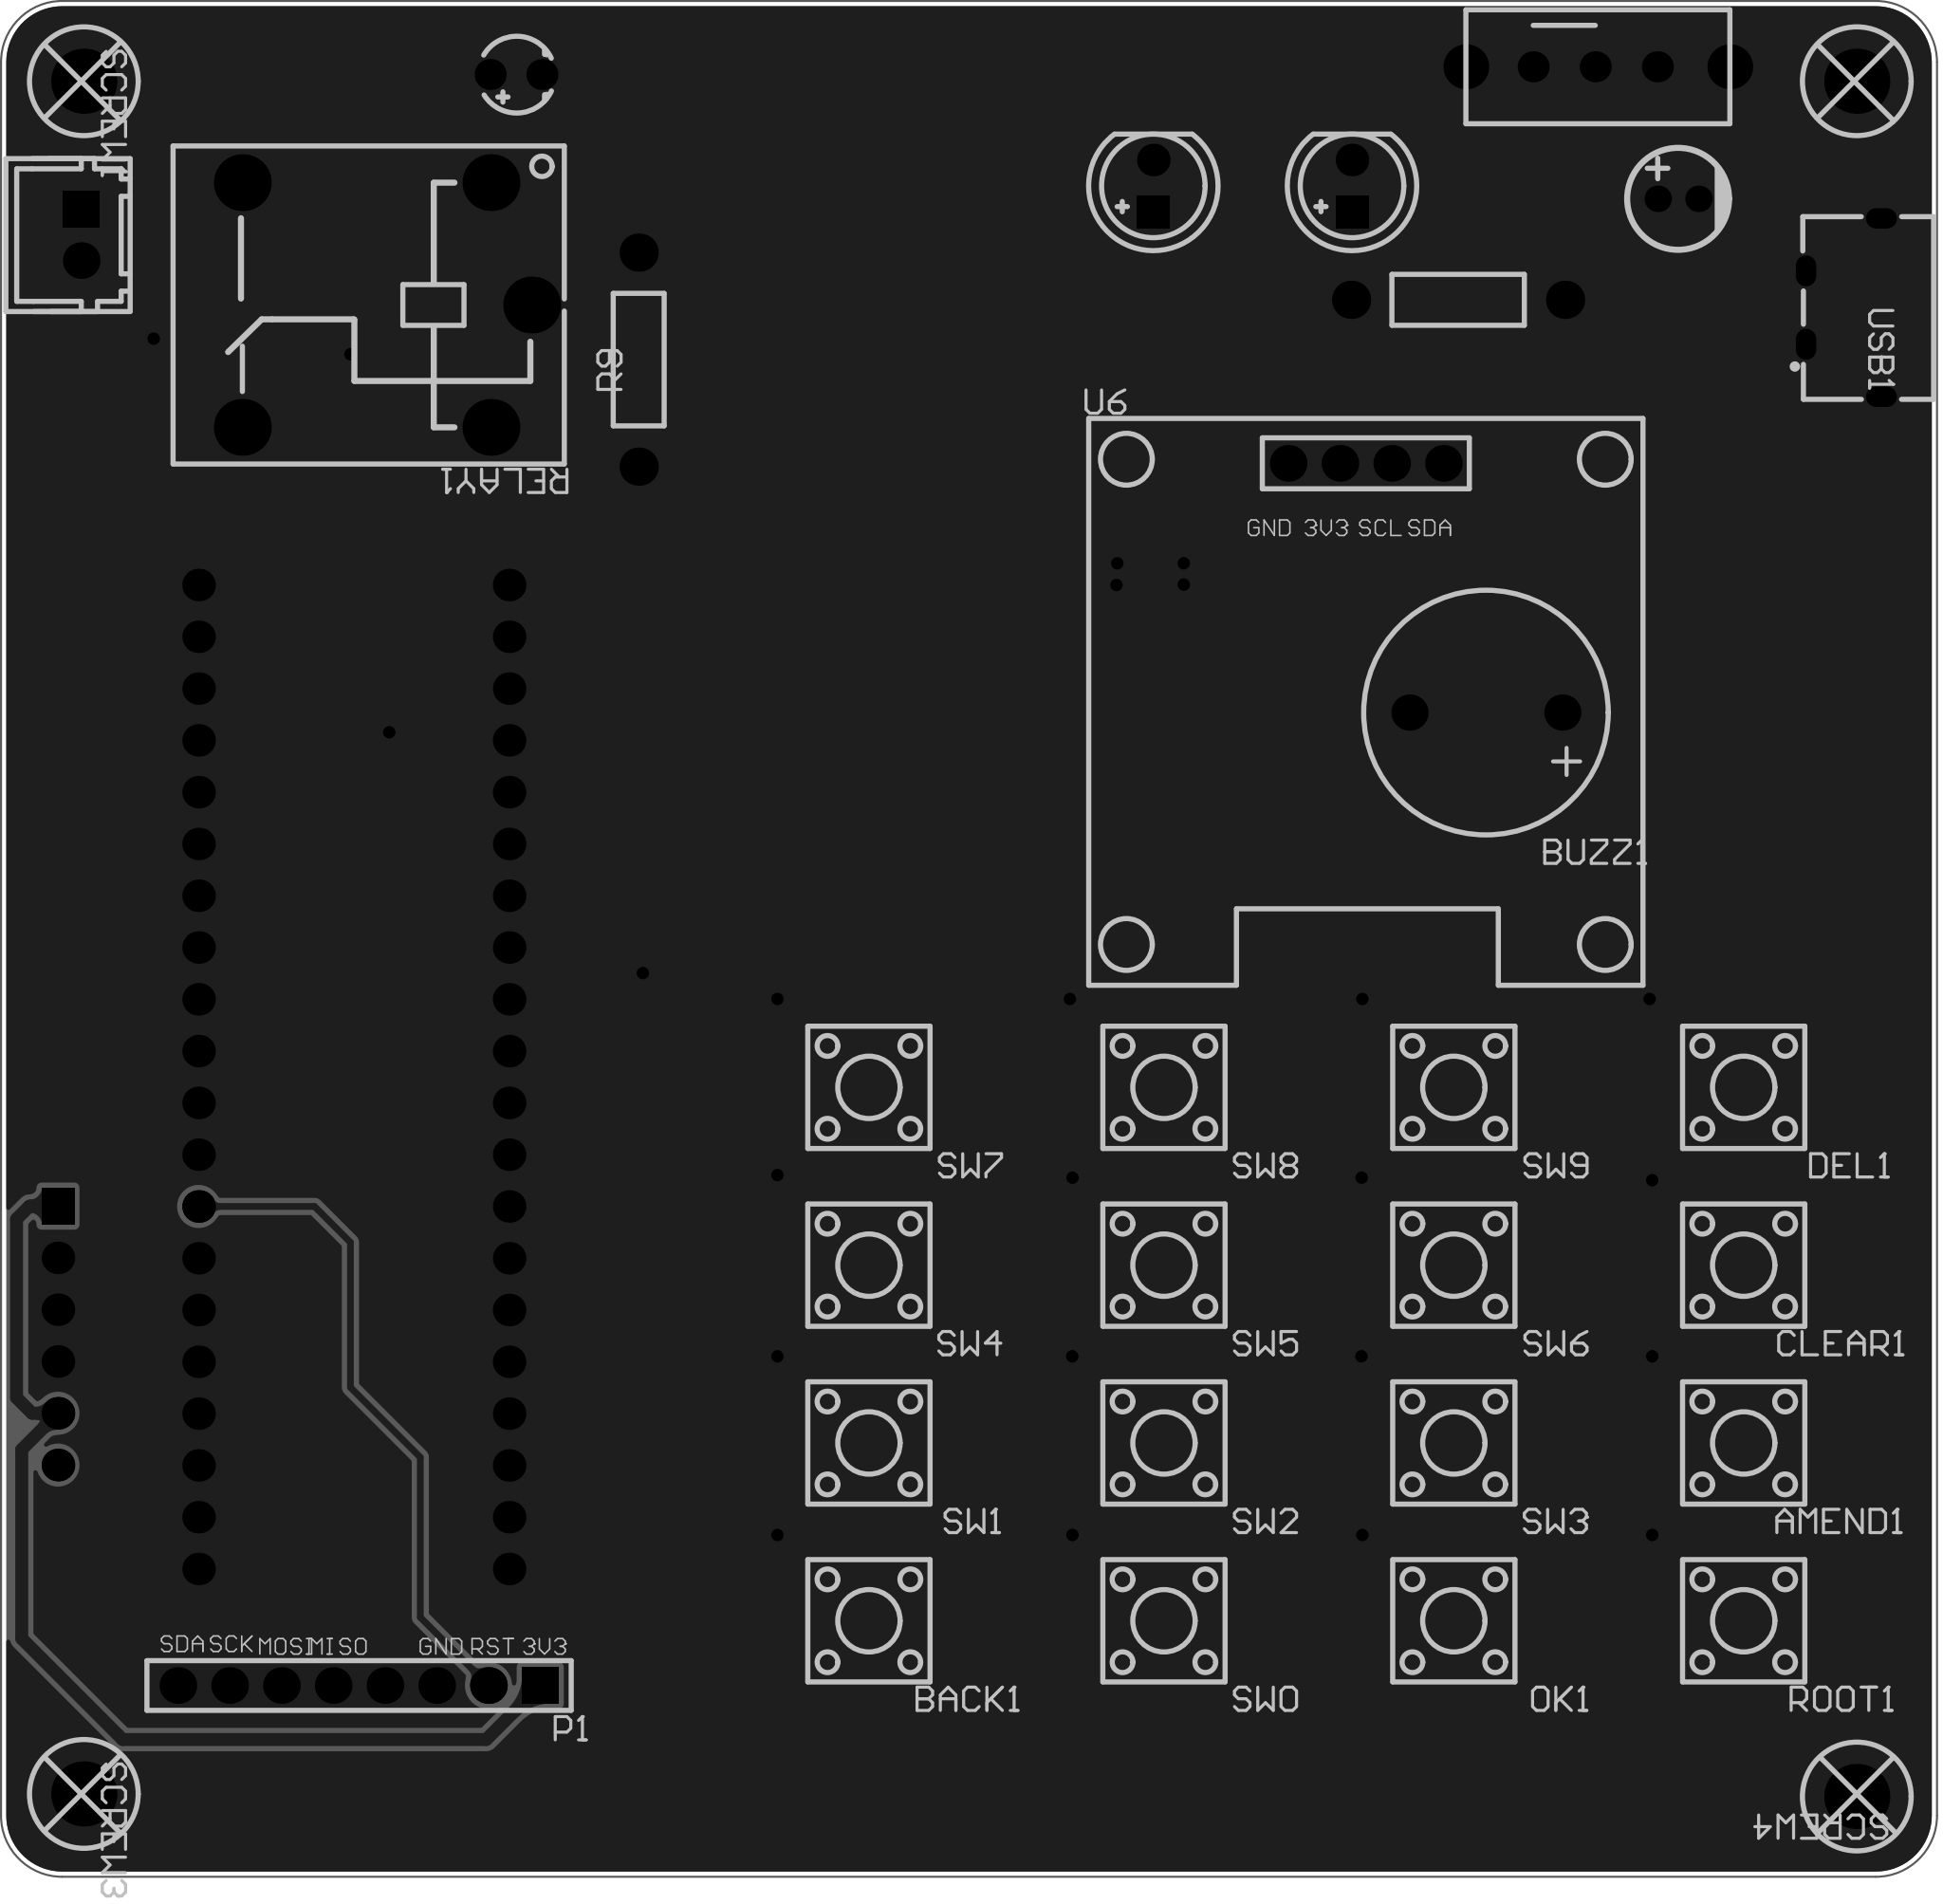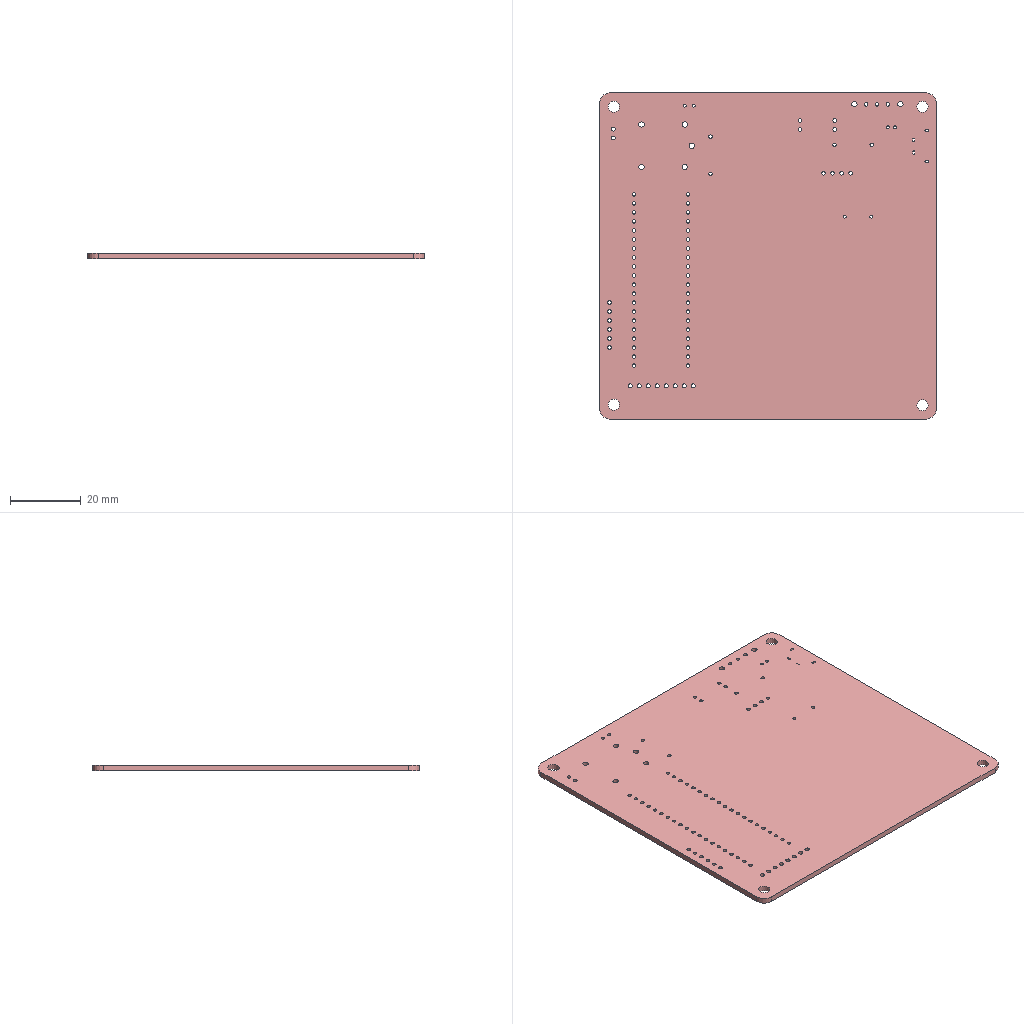Circuit board layout | Altium Designer | box 95 x 92 x 1.6 mm
Layer stack:
# Altium Designer layer stack of  (unit mm; dielectric type: 0 none, 1 core, 2 prepreg, 3 surface material)
index,name,kind,layer,copper_thickness_mm,dielectric_type,dielectric_thickness_mm,dielectric_material,dielectric_constant
0,Top Paste Mask Layer,other,,,,,,
1,Top Silkscreen Layer,other,,,,,,
2,Top Solder Mask Layer,dielectric,,,3,0.01,,3.3
3,Top Layer,copper,Top Layer,0.035,,,,
4,Dielectric1,dielectric,,,3,1.51,FR4,4.5
5,Bottom Layer,copper,Bottom Layer,0.035,,,,
6,Bottom Solder Mask Layer,dielectric,,,3,0.01,,3.3
7,Bottom Silkscreen Layer,other,,,,,,
8,Bottom Paste Mask Layer,other,,,,,,
# drill layer pairs: low layer,high layer
drill_pair,Top Layer,Bottom Layer
Part placement:
Designator,Comment,Layer,Footprint,Center-X(mm),Center-Y(mm),Rotation
BUZZ1,Buzzer BD12.0-P7.50,TopLayer,BUZ-TH_BD12.0-P7.50-D0.6-FD,150.464,138,180
U7,STM32F103C8T6-Card,BottomLayer,CONN-TH_L53.3-W22.9_STM32F103C8T6-CARD,94.912,120.125,90
CN1,ZX-XH2.54-2PZZ,TopLayer,CONN-TH_2P-P2.50_HX25003-2A,81.534,161.417,270
D1,SS14,BottomLayer,SMA_L4.2-W2.6-LS5.3-RD,97.574,154.567,270
RELAY1,SRD-12VDC-SL-C,TopLayer,RELAY-TH_SRD-XXVDC-XL-C,96.539,157.989,180
R1,10.1kΩ,BottomLayer,R0805,126.619,157.837,0
Q1,S8050,BottomLayer,SOT-23-3_L2.9-W1.6-P1.90-LS2.8-BR,93.764,153.17,90
R6,1kΩ,BottomLayer,R0603,92.761,157.107,90
U6,HS96L03W2C03,TopLayer,OLED-TH_L27.8-W27.2-P2.54_C9900033791,144.569,150.224,0
H2,PM254V-11-06-H85,BottomLayer,hdr-th_6p-p2.54-v-f,80.391,107.442,270
P1,2.54-1*8P female, RoHS,TopLayer,HDR-TH_8P-P2.54-V-F-1,95.166,90.28,180
SW8,KH-6X6X5H-STM,TopLayer,SW-SMD_4P-L6.0-W6.0-P4.50-LS9.0-2,134.663,119.617,180
SW5,KH-6X6X5H-STM,TopLayer,SW-SMD_4P-L6.0-W6.0-P4.50-LS9.0-2,134.663,110.896,180
SW2,KH-6X6X5H-STM,TopLayer,SW-SMD_4P-L6.0-W6.0-P4.50-LS9.0-2,134.663,102.176,180
OK1,KH-6X6X5H-STM,TopLayer,SW-SMD_4P-L6.0-W6.0-P4.50-LS9.0-2,148.887,93.455,180
BACK1,KH-6X6X5H-STM,TopLayer,SW-SMD_4P-L6.0-W6.0-P4.50-LS9.0-2,120.185,93.455,180
AMEND1,KH-6X6X5H-STM,TopLayer,SW-SMD_4P-L6.0-W6.0-P4.50-LS9.0-2,163.111,102.176,180
SW7,KH-6X6X5H-STM,TopLayer,SW-SMD_4P-L6.0-W6.0-P4.50-LS9.0-2,120.185,119.617,180
SW4,KH-6X6X5H-STM,TopLayer,SW-SMD_4P-L6.0-W6.0-P4.50-LS9.0-2,120.185,110.896,180
SW9,KH-6X6X5H-STM,TopLayer,SW-SMD_4P-L6.0-W6.0-P4.50-LS9.0-2,148.887,119.617,180
SW6,KH-6X6X5H-STM,TopLayer,SW-SMD_4P-L6.0-W6.0-P4.50-LS9.0-2,148.887,110.896,180
SW1,KH-6X6X5H-STM,TopLayer,SW-SMD_4P-L6.0-W6.0-P4.50-LS9.0-2,120.185,102.176,180
SW3,KH-6X6X5H-STM,TopLayer,SW-SMD_4P-L6.0-W6.0-P4.50-LS9.0-2,148.887,102.176,180
SW0,KH-6X6X5H-STM,TopLayer,SW-SMD_4P-L6.0-W6.0-P4.50-LS9.0-2,134.663,93.455,180
CLEAR1,KH-6X6X5H-STM,TopLayer,SW-SMD_4P-L6.0-W6.0-P4.50-LS9.0-2,163.111,110.896,180
DEL1,KH-6X6X5H-STM,TopLayer,SW-SMD_4P-L6.0-W6.0-P4.50-LS9.0-2,163.111,119.617,180
ROOT1,KH-6X6X5H-STM,TopLayer,SW-SMD_4P-L6.0-W6.0-P4.50-LS9.0-2,163.111,93.455,180
U8,AT24C02,BottomLayer,SOP-8_L5.0-W4.0-P1.27-LS6.0-BL,93.903,133.35,270
USB1,KH-TYPE-C-2P,TopLayer,USB-SMD_KH-TYPE-C-2P,168.021,157.861,90
SW10,SK-12E12-G5,TopLayer,SW-TH_SK-12E12-G5,155.956,169.672,90
R8,1kΩ,TopLayer,RES-TH_BD2.5-L6.5-P10.50-D0.6,149.098,158.242,180
C10,10uF,TopLayer,CAP-TH_BD5.0-P2.00-D0.8-FD,159.893,163.195,0
C11,1uF,BottomLayer,C0603,126.252,164.202,270
C12,1uF,BottomLayer,C0603,116.459,158.488,270
C13,100nF,BottomLayer,C0603,128.524,164.202,270
C14,100nF,BottomLayer,C0603,114.173,158.488,270
U9,AMS1117-3.3,BottomLayer,SOT-223-4_L6.5-W3.5-P2.30-LS7.0-BR,121.512,160.649,90
SCREW1,,TopLayer,M3螺丝,81.66,168.963,270
SCREW2,,TopLayer,M3螺丝,168.661,168.963,270
SCREW3,,TopLayer,M3螺丝,81.66,84.963,270
SCREW4,,TopLayer,M3螺丝,168.661,84.835,180
LED5,XL-302SURD,TopLayer,LED-TH_BD3.8-P2.54-RD,102.87,169.291,180
R9,1kΩ,TopLayer,RES-TH_BD2.5-L6.5-P10.50-D0.6,108.888,155.31,90
LED2,,TopLayer,LED-TH_5mm,134.142,163.83,90
LED6,,TopLayer,LED-TH_5mm,143.891,163.83,90
Pad and via stacks:
# Altium Designer via and pad stacks of  (unit mm). Each distinct definition once, with the count of objects using it.
# via: kind,start_layer,end_layer,hole_mm,diameter_mm,mode(0 simple;1 top-mid-bottom;2 full stack),diameter_per_layer,count,example_net
# pad: kind,layer,hole_mm,hole_type(0 round;1 square;2 slot),plating,top_size,top_shape(1 round;2 rect;3 octagon;9 rounded rect),mid_size,bottom_size,mode,footprint,size_per_layer,count,example
pad,Multi-Layer,0.9,0,plated,1.778x1.778,1,1.778x1.778,1.778x1.778,0,BUZ-TH_BD12.0-P7.50-D0.6-FD,,2,BUZZ1.2
pad,Multi-Layer,1,0,plated,1.6x1.6,1,1.6x1.6,1.6x1.6,0,CONN-TH_L53.3-W22.9_STM32F103C8T6-CARD,,40,U7.1
pad,Multi-Layer,1.1,0,plated,1.8x1.8,2,1.8x1.8,1.8x1.8,0,CONN-TH_2P-P2.50_HX25003-2A,,1,CN1.1
pad,Multi-Layer,1.1,0,plated,1.8x1.8,1,1.8x1.8,1.8x1.8,0,CONN-TH_2P-P2.50_HX25003-2A,,1,CN1.2
pad,Multi-Layer,1.524,0,plated,2.794x2.794,1,2.794x2.794,2.794x2.794,0,RELAY-TH_SRD-XXVDC-XL-C,,5,RELAY1.2
pad,Multi-Layer,1.05,0,plated,1.8x1.8,1,1.8x1.8,1.8x1.8,0,OLED-TH_L27.8-W27.2-P2.54_C9900033791,,4,U6.1
pad,Multi-Layer,1.02,0,plated,1.6x1.6,1,1.6x1.6,1.6x1.6,0,hdr-th_6p-p2.54-v-f,,5,H2.6
pad,Multi-Layer,1.02,0,plated,1.8x1.6,2,1.8x1.6,1.8x1.6,0,hdr-th_6p-p2.54-v-f,,1,H2.1
pad,Multi-Layer,1.2,0,plated,1.8x1.8,2,1.8x1.8,1.8x1.8,0,HDR-TH_8P-P2.54-V-F-1,,1,P1.1
pad,Multi-Layer,1.2,0,plated,1.8x1.8,1,1.8x1.8,1.8x1.8,0,HDR-TH_8P-P2.54-V-F-1,,7,P1.2
pad,Multi-Layer,0.45,2,plated,1x1.524,1,1x1.524,1x1.524,0,USB-SMD_KH-TYPE-C-2P,,2,USB1.1
pad,Multi-Layer,0.5,2,plated,1x1.524,1,1x1.524,1x1.524,0,USB-SMD_KH-TYPE-C-2P,,2,USB1.3
pad,Multi-Layer,1,0,plated,1.524x1.524,1,1.524x1.524,1.524x1.524,0,SW-TH_SK-12E12-G5,,3,SW10.2
pad,Multi-Layer,1.5,0,plated,2.2x2.2,1,2.2x2.2,2.2x2.2,0,SW-TH_SK-12E12-G5,,2,SW10.4
pad,Multi-Layer,1,0,plated,1.88x1.88,1,1.88x1.88,1.88x1.88,0,RES-TH_BD2.5-L6.5-P10.50-D0.6,,4,R8.1
pad,Multi-Layer,0.8,0,plated,1.3x1.3,1,1.3x1.3,1.3x1.3,0,CAP-TH_BD5.0-P2.00-D0.8-FD,,2,C10.1
pad,Multi-Layer,3.2,0,plated,3.2x3.2,1,3.2x3.2,3.2x3.2,0,M3\u00C2\u00DD\u00CB\u00BF,,4,SCREW1.1
pad,Multi-Layer,0.9,0,plated,1.524x1.524,1,1.524x1.524,1.524x1.524,0,LED-TH_BD3.8-P2.54-RD,,2,LED5.2
pad,Multi-Layer,1,0,plated,1.6x1.6,2,1.6x1.6,1.6x1.6,0,LED-TH_5mm,,2,LED2.1
pad,Multi-Layer,1,0,plated,1.6x1.6,1,1.6x1.6,1.6x1.6,0,LED-TH_5mm,,2,LED2.2
pad,Bottom Layer,0,0,plated,2.2x1.7,2,2.2x1.7,2.2x1.7,0,SMA_L4.2-W2.6-LS5.3-RD,,2,D1.1
pad,Bottom Layer,0,0,plated,1.133x1.377,2,1.133x1.377,1.133x1.377,0,R0805,,2,R1.2
pad,Bottom Layer,0,0,plated,1.07x0.6,2,1.07x0.6,1.07x0.6,0,SOT-23-3_L2.9-W1.6-P1.90-LS2.8-BR,,3,Q1.1
pad,Bottom Layer,0,0,plated,0.8065x0.864,2,0.8065x0.864,0.8065x0.864,0,R0603,,2,R6.2
pad,Bottom Layer,0,0,plated,0.574x2.035,1,0.574x2.035,0.574x2.035,0,SOP-8_L5.0-W4.0-P1.27-LS6.0-BL,,8,U8.1
pad,Bottom Layer,0,0,plated,0.8x0.9,2,0.8x0.9,0.8x0.9,0,C0603,,8,C11.2
pad,Bottom Layer,0,0,plated,2.47x0.98,2,2.47x0.98,2.47x0.98,0,SOT-223-4_L6.5-W3.5-P2.30-LS7.0-BR,,3,U9.1
pad,Bottom Layer,0,0,plated,2.47x3.6,2,2.47x3.6,2.47x3.6,0,SOT-223-4_L6.5-W3.5-P2.30-LS7.0-BR,,1,U9.4
pad,Top Layer,0,0,plated,2.3x1.5,2,2.3x1.5,2.3x1.5,0,SW-SMD_4P-L6.0-W6.0-P4.50-LS9.0-2,,64,SW8.1
via,Top Layer,Bottom Layer,0.3048,0.6096,0,,24,KEY5
Copper pours:
name,layer,net,type(0 solid;1 hatched;2 none)
Top Layer-GND,Top Layer,GND,0
Bottom Layer-GND,Bottom Layer,GND,0
Design rules, without the lines most boards share:
# Altium Designer design rules of  (exported by Altium Designer, unit mm)
# columns: name | kind | enabled | priority | scope1 | scope2 | descriptor | typed fields (field=value)
copperThickness2oz | 0 | disabled | 1 | All | All | Clearance Constraint (Gap=6mil) (Disabled)(All),(All) | gap=0.1524
Plane_innerPlane | 0 | disabled | 2 | All | All | Clearance Constraint (Gap=6mil) (Disabled)(All),(All) | gap=0.1524
Copper_copperRegion | 0 | disabled | 3 | All | All | Clearance Constraint (Gap=6mil) (Disabled)(All),(All) | gap=0.1524
copperThickness1oz | 0 | enabled | 4 | All | All | Clearance Constraint (Gap=6mil) (All),(All) | gap=0.1524
otherClearance | 52 | enabled | 1 | All | All | Hole To Hole Clearance (Gap=11.8mil) (All),(All) | gap=0.2997
copperThickness2oz_2 | 2 | enabled | 1 | (InNet('+3V3') OR InNet('+5V') OR InNet('GND')) | All | Width Constraint (Min=8mil) (Max=100mil) (Preferred=25mil) ((InNet('+3V3') OR InNet('+5V') OR InNet('GND'))) |
copperThickness1oz_2 | 2 | enabled | 2 | All | All | Width Constraint (Min=5mil) (Max=100mil) (Preferred=13mil) (All) |
viaSize | 11 | enabled | 1 | All | All | Routing Via (MinHoleWidth=11.8mil) (MaxHoleWidth=248mil) (PreferredHoleWidth=12mil) (MinWidth=19.7mil) (MaxWidth=393.7mil) (PreferedWidth=24mil) (All) | via_min_hole=0.2997 via_max_hole=6.299 via_preferred_diameter=0.6096 via_preferred_hole=0.3048